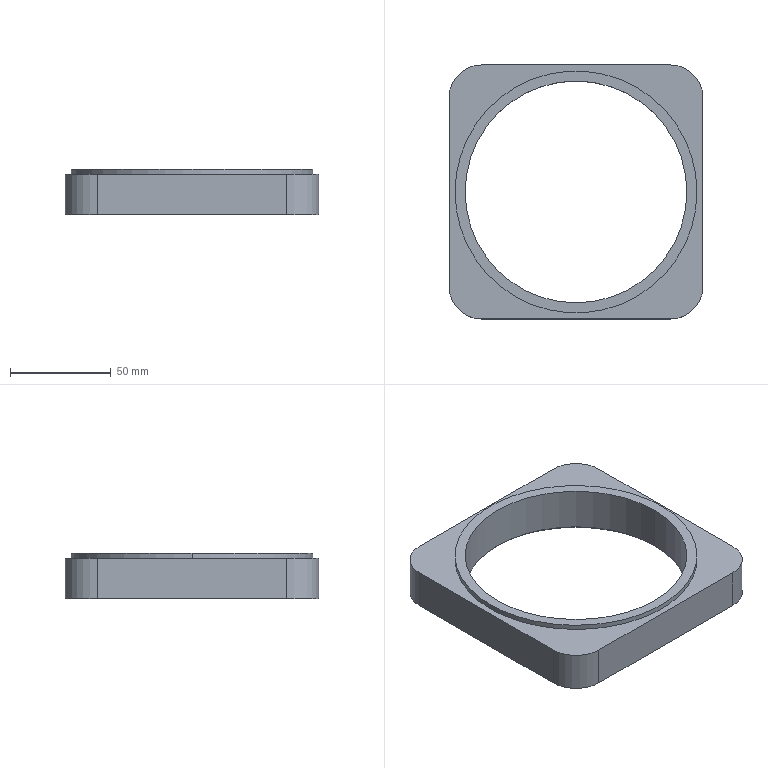Part | SolidWorks | features 3DProfileFeature 1, Chamfer 1, Extrusion 1, HoleWzd 1, ICE 1 | 1 solid | 33 faces | box 126 x 126 x 22.5 mm | volume 124484 mm3 | cylinder 16 | cone 10 | plane 7 | commonest cylinder face diameters 8.5 x8 32 x4 110 x2 120 x2
STEP:
#1=CARTESIAN_POINT('',(118.,63.,1.));
#2=VERTEX_POINT('',#1);
#3=CARTESIAN_POINT('',(8.,63.,1.));
#4=VERTEX_POINT('',#3);
#5=CARTESIAN_POINT('',(63.,63.,1.));
#6=DIRECTION('',(0.,0.,-1.));
#7=DIRECTION('',(1.,0.,0.));
#8=AXIS2_PLACEMENT_3D('',#5,#6,#7);
#9=CIRCLE('',#8,55.);
#10=EDGE_CURVE('',#2,#4,#9,.T.);
#11=ORIENTED_EDGE('',*,*,#10,.F.);
#12=CARTESIAN_POINT('',(119.,63.,0.));
#13=VERTEX_POINT('',#12);
#14=CARTESIAN_POINT('',(119.,63.,0.));
#15=DIRECTION('',(0.7071,0.,-0.7071));
#16=VECTOR('',#15,1000.);
#17=LINE('',#14,#16);
#18=EDGE_CURVE('',#2,#13,#17,.T.);
#19=ORIENTED_EDGE('',*,*,#18,.T.);
#20=CARTESIAN_POINT('',(7.,63.,0.));
#21=VERTEX_POINT('',#20);
#22=CARTESIAN_POINT('',(63.,63.,0.));
#23=DIRECTION('',(0.,0.,1.));
#24=DIRECTION('',(1.,0.,0.));
#25=AXIS2_PLACEMENT_3D('',#22,#23,#24);
#26=CIRCLE('',#25,56.);
#27=EDGE_CURVE('',#21,#13,#26,.T.);
#28=ORIENTED_EDGE('',*,*,#27,.F.);
#29=CARTESIAN_POINT('',(7.,63.,0.));
#30=DIRECTION('',(-0.7071,0.,-0.7071));
#31=VECTOR('',#30,1000.);
#32=LINE('',#29,#31);
#33=EDGE_CURVE('',#4,#21,#32,.T.);
#34=ORIENTED_EDGE('',*,*,#33,.F.);
#35=EDGE_LOOP('',(#11,#19,#28,#34));
#36=FACE_OUTER_BOUND('',#35,.T.);
#37=CARTESIAN_POINT('',(63.,63.,0.));
#38=DIRECTION('',(0.,0.,-1.));
#39=DIRECTION('',(-1.,0.,0.));
#40=AXIS2_PLACEMENT_3D('',#37,#38,#39);
#41=CONICAL_SURFACE('',#40,56.,0.7854);
#42=ADVANCED_FACE('',(#36),#41,.F.);
#43=CARTESIAN_POINT('',(114.25,110.,12.));
#44=VERTEX_POINT('',#43);
#45=CARTESIAN_POINT('',(105.75,110.,12.));
#46=VERTEX_POINT('',#45);
#47=CARTESIAN_POINT('',(110.,110.,12.));
#48=DIRECTION('',(0.,0.,-1.));
#49=DIRECTION('',(-1.,0.,0.));
#50=AXIS2_PLACEMENT_3D('',#47,#48,#49);
#51=CIRCLE('',#50,4.25);
#52=EDGE_CURVE('',#44,#46,#51,.T.);
#53=ORIENTED_EDGE('',*,*,#52,.F.);
#54=CARTESIAN_POINT('',(114.25,110.,0.));
#55=VERTEX_POINT('',#54);
#56=CARTESIAN_POINT('',(114.25,110.,0.));
#57=DIRECTION('',(0.,0.,-1.));
#58=VECTOR('',#57,1000.);
#59=LINE('',#56,#58);
#60=EDGE_CURVE('',#44,#55,#59,.T.);
#61=ORIENTED_EDGE('',*,*,#60,.T.);
#62=CARTESIAN_POINT('',(105.75,110.,0.));
#63=VERTEX_POINT('',#62);
#64=CARTESIAN_POINT('',(110.,110.,0.));
#65=DIRECTION('',(0.,0.,-1.));
#66=DIRECTION('',(-1.,0.,0.));
#67=AXIS2_PLACEMENT_3D('',#64,#65,#66);
#68=CIRCLE('',#67,4.25);
#69=EDGE_CURVE('',#55,#63,#68,.T.);
#70=ORIENTED_EDGE('',*,*,#69,.T.);
#71=CARTESIAN_POINT('',(105.75,110.,0.));
#72=DIRECTION('',(0.,0.,-1.));
#73=VECTOR('',#72,1000.);
#74=LINE('',#71,#73);
#75=EDGE_CURVE('',#46,#63,#74,.T.);
#76=ORIENTED_EDGE('',*,*,#75,.F.);
#77=EDGE_LOOP('',(#53,#61,#70,#76));
#78=FACE_OUTER_BOUND('',#77,.T.);
#79=CARTESIAN_POINT('',(110.,110.,0.));
#80=DIRECTION('',(0.,0.,-1.));
#81=DIRECTION('',(-1.,0.,0.));
#82=AXIS2_PLACEMENT_3D('',#79,#80,#81);
#83=CYLINDRICAL_SURFACE('',#82,4.25);
#84=ADVANCED_FACE('',(#78),#83,.F.);
#85=CARTESIAN_POINT('',(110.,110.,14.554));
#86=VERTEX_POINT('',#85);
#87=CARTESIAN_POINT('',(105.75,110.,12.));
#88=DIRECTION('',(-0.8572,0.,-0.515));
#89=VECTOR('',#88,1000.);
#90=LINE('',#87,#89);
#91=EDGE_CURVE('',#86,#46,#90,.T.);
#92=ORIENTED_EDGE('',*,*,#91,.F.);
#93=CARTESIAN_POINT('',(114.25,110.,12.));
#94=DIRECTION('',(0.8572,0.,-0.515));
#95=VECTOR('',#94,1000.);
#96=LINE('',#93,#95);
#97=EDGE_CURVE('',#86,#44,#96,.T.);
#98=ORIENTED_EDGE('',*,*,#97,.T.);
#99=ORIENTED_EDGE('',*,*,#52,.T.);
#100=EDGE_LOOP('',(#92,#98,#99));
#101=FACE_OUTER_BOUND('',#100,.T.);
#102=CARTESIAN_POINT('',(110.,110.,12.));
#103=DIRECTION('',(0.,0.,-1.));
#104=DIRECTION('',(-1.,0.,0.));
#105=AXIS2_PLACEMENT_3D('',#102,#103,#104);
#106=CONICAL_SURFACE('',#105,4.25,1.03);
#107=ADVANCED_FACE('',(#101),#106,.F.);
#108=CARTESIAN_POINT('',(20.25,110.,12.));
#109=VERTEX_POINT('',#108);
#110=CARTESIAN_POINT('',(11.75,110.,12.));
#111=VERTEX_POINT('',#110);
#112=CARTESIAN_POINT('',(16.,110.,12.));
#113=DIRECTION('',(0.,0.,-1.));
#114=DIRECTION('',(-1.,0.,0.));
#115=AXIS2_PLACEMENT_3D('',#112,#113,#114);
#116=CIRCLE('',#115,4.25);
#117=EDGE_CURVE('',#109,#111,#116,.T.);
#118=ORIENTED_EDGE('',*,*,#117,.F.);
#119=CARTESIAN_POINT('',(20.25,110.,0.));
#120=VERTEX_POINT('',#119);
#121=CARTESIAN_POINT('',(20.25,110.,0.));
#122=DIRECTION('',(0.,0.,-1.));
#123=VECTOR('',#122,1000.);
#124=LINE('',#121,#123);
#125=EDGE_CURVE('',#109,#120,#124,.T.);
#126=ORIENTED_EDGE('',*,*,#125,.T.);
#127=CARTESIAN_POINT('',(11.75,110.,0.));
#128=VERTEX_POINT('',#127);
#129=CARTESIAN_POINT('',(16.,110.,0.));
#130=DIRECTION('',(0.,0.,-1.));
#131=DIRECTION('',(-1.,0.,0.));
#132=AXIS2_PLACEMENT_3D('',#129,#130,#131);
#133=CIRCLE('',#132,4.25);
#134=EDGE_CURVE('',#120,#128,#133,.T.);
#135=ORIENTED_EDGE('',*,*,#134,.T.);
#136=CARTESIAN_POINT('',(11.75,110.,0.));
#137=DIRECTION('',(0.,0.,-1.));
#138=VECTOR('',#137,1000.);
#139=LINE('',#136,#138);
#140=EDGE_CURVE('',#111,#128,#139,.T.);
#141=ORIENTED_EDGE('',*,*,#140,.F.);
#142=EDGE_LOOP('',(#118,#126,#135,#141));
#143=FACE_OUTER_BOUND('',#142,.T.);
#144=CARTESIAN_POINT('',(16.,110.,0.));
#145=DIRECTION('',(0.,0.,-1.));
#146=DIRECTION('',(-1.,0.,0.));
#147=AXIS2_PLACEMENT_3D('',#144,#145,#146);
#148=CYLINDRICAL_SURFACE('',#147,4.25);
#149=ADVANCED_FACE('',(#143),#148,.F.);
#150=CARTESIAN_POINT('',(16.,110.,14.554));
#151=VERTEX_POINT('',#150);
#152=CARTESIAN_POINT('',(11.75,110.,12.));
#153=DIRECTION('',(-0.8572,0.,-0.515));
#154=VECTOR('',#153,1000.);
#155=LINE('',#152,#154);
#156=EDGE_CURVE('',#151,#111,#155,.T.);
#157=ORIENTED_EDGE('',*,*,#156,.F.);
#158=CARTESIAN_POINT('',(20.25,110.,12.));
#159=DIRECTION('',(0.8572,0.,-0.515));
#160=VECTOR('',#159,1000.);
#161=LINE('',#158,#160);
#162=EDGE_CURVE('',#151,#109,#161,.T.);
#163=ORIENTED_EDGE('',*,*,#162,.T.);
#164=ORIENTED_EDGE('',*,*,#117,.T.);
#165=EDGE_LOOP('',(#157,#163,#164));
#166=FACE_OUTER_BOUND('',#165,.T.);
#167=CARTESIAN_POINT('',(16.,110.,12.));
#168=DIRECTION('',(0.,0.,-1.));
#169=DIRECTION('',(-1.,0.,0.));
#170=AXIS2_PLACEMENT_3D('',#167,#168,#169);
#171=CONICAL_SURFACE('',#170,4.25,1.03);
#172=ADVANCED_FACE('',(#166),#171,.F.);
#173=CARTESIAN_POINT('',(20.25,16.,12.));
#174=VERTEX_POINT('',#173);
#175=CARTESIAN_POINT('',(11.75,16.,12.));
#176=VERTEX_POINT('',#175);
#177=CARTESIAN_POINT('',(16.,16.,12.));
#178=DIRECTION('',(0.,0.,-1.));
#179=DIRECTION('',(-1.,0.,0.));
#180=AXIS2_PLACEMENT_3D('',#177,#178,#179);
#181=CIRCLE('',#180,4.25);
#182=EDGE_CURVE('',#174,#176,#181,.T.);
#183=ORIENTED_EDGE('',*,*,#182,.F.);
#184=CARTESIAN_POINT('',(20.25,16.,0.));
#185=VERTEX_POINT('',#184);
#186=CARTESIAN_POINT('',(20.25,16.,0.));
#187=DIRECTION('',(0.,0.,-1.));
#188=VECTOR('',#187,1000.);
#189=LINE('',#186,#188);
#190=EDGE_CURVE('',#174,#185,#189,.T.);
#191=ORIENTED_EDGE('',*,*,#190,.T.);
#192=CARTESIAN_POINT('',(11.75,16.,0.));
#193=VERTEX_POINT('',#192);
#194=CARTESIAN_POINT('',(16.,16.,0.));
#195=DIRECTION('',(0.,0.,-1.));
#196=DIRECTION('',(-1.,0.,0.));
#197=AXIS2_PLACEMENT_3D('',#194,#195,#196);
#198=CIRCLE('',#197,4.25);
#199=EDGE_CURVE('',#185,#193,#198,.T.);
#200=ORIENTED_EDGE('',*,*,#199,.T.);
#201=CARTESIAN_POINT('',(11.75,16.,0.));
#202=DIRECTION('',(0.,0.,-1.));
#203=VECTOR('',#202,1000.);
#204=LINE('',#201,#203);
#205=EDGE_CURVE('',#176,#193,#204,.T.);
#206=ORIENTED_EDGE('',*,*,#205,.F.);
#207=EDGE_LOOP('',(#183,#191,#200,#206));
#208=FACE_OUTER_BOUND('',#207,.T.);
#209=CARTESIAN_POINT('',(16.,16.,0.));
#210=DIRECTION('',(0.,0.,-1.));
#211=DIRECTION('',(-1.,0.,0.));
#212=AXIS2_PLACEMENT_3D('',#209,#210,#211);
#213=CYLINDRICAL_SURFACE('',#212,4.25);
#214=ADVANCED_FACE('',(#208),#213,.F.);
#215=CARTESIAN_POINT('',(16.,16.,14.554));
#216=VERTEX_POINT('',#215);
#217=CARTESIAN_POINT('',(11.75,16.,12.));
#218=DIRECTION('',(-0.8572,0.,-0.515));
#219=VECTOR('',#218,1000.);
#220=LINE('',#217,#219);
#221=EDGE_CURVE('',#216,#176,#220,.T.);
#222=ORIENTED_EDGE('',*,*,#221,.F.);
#223=CARTESIAN_POINT('',(20.25,16.,12.));
#224=DIRECTION('',(0.8572,0.,-0.515));
#225=VECTOR('',#224,1000.);
#226=LINE('',#223,#225);
#227=EDGE_CURVE('',#216,#174,#226,.T.);
#228=ORIENTED_EDGE('',*,*,#227,.T.);
#229=ORIENTED_EDGE('',*,*,#182,.T.);
#230=EDGE_LOOP('',(#222,#228,#229));
#231=FACE_OUTER_BOUND('',#230,.T.);
#232=CARTESIAN_POINT('',(16.,16.,12.));
#233=DIRECTION('',(0.,0.,-1.));
#234=DIRECTION('',(-1.,0.,0.));
#235=AXIS2_PLACEMENT_3D('',#232,#233,#234);
#236=CONICAL_SURFACE('',#235,4.25,1.03);
#237=ADVANCED_FACE('',(#231),#236,.F.);
#238=CARTESIAN_POINT('',(114.25,16.,12.));
#239=VERTEX_POINT('',#238);
#240=CARTESIAN_POINT('',(105.75,16.,12.));
#241=VERTEX_POINT('',#240);
#242=CARTESIAN_POINT('',(110.,16.,12.));
#243=DIRECTION('',(0.,0.,-1.));
#244=DIRECTION('',(-1.,0.,0.));
#245=AXIS2_PLACEMENT_3D('',#242,#243,#244);
#246=CIRCLE('',#245,4.25);
#247=EDGE_CURVE('',#239,#241,#246,.T.);
#248=ORIENTED_EDGE('',*,*,#247,.F.);
#249=CARTESIAN_POINT('',(114.25,16.,0.));
#250=VERTEX_POINT('',#249);
#251=CARTESIAN_POINT('',(114.25,16.,0.));
#252=DIRECTION('',(0.,0.,-1.));
#253=VECTOR('',#252,1000.);
#254=LINE('',#251,#253);
#255=EDGE_CURVE('',#239,#250,#254,.T.);
#256=ORIENTED_EDGE('',*,*,#255,.T.);
#257=CARTESIAN_POINT('',(105.75,16.,0.));
#258=VERTEX_POINT('',#257);
#259=CARTESIAN_POINT('',(110.,16.,0.));
#260=DIRECTION('',(0.,0.,-1.));
#261=DIRECTION('',(-1.,0.,0.));
#262=AXIS2_PLACEMENT_3D('',#259,#260,#261);
#263=CIRCLE('',#262,4.25);
#264=EDGE_CURVE('',#250,#258,#263,.T.);
#265=ORIENTED_EDGE('',*,*,#264,.T.);
#266=CARTESIAN_POINT('',(105.75,16.,0.));
#267=DIRECTION('',(0.,0.,-1.));
#268=VECTOR('',#267,1000.);
#269=LINE('',#266,#268);
#270=EDGE_CURVE('',#241,#258,#269,.T.);
#271=ORIENTED_EDGE('',*,*,#270,.F.);
#272=EDGE_LOOP('',(#248,#256,#265,#271));
#273=FACE_OUTER_BOUND('',#272,.T.);
#274=CARTESIAN_POINT('',(110.,16.,0.));
#275=DIRECTION('',(0.,0.,-1.));
#276=DIRECTION('',(-1.,0.,0.));
#277=AXIS2_PLACEMENT_3D('',#274,#275,#276);
#278=CYLINDRICAL_SURFACE('',#277,4.25);
#279=ADVANCED_FACE('',(#273),#278,.F.);
#280=CARTESIAN_POINT('',(110.,16.,14.554));
#281=VERTEX_POINT('',#280);
#282=CARTESIAN_POINT('',(105.75,16.,12.));
#283=DIRECTION('',(-0.8572,0.,-0.515));
#284=VECTOR('',#283,1000.);
#285=LINE('',#282,#284);
#286=EDGE_CURVE('',#281,#241,#285,.T.);
#287=ORIENTED_EDGE('',*,*,#286,.F.);
#288=CARTESIAN_POINT('',(114.25,16.,12.));
#289=DIRECTION('',(0.8572,0.,-0.515));
#290=VECTOR('',#289,1000.);
#291=LINE('',#288,#290);
#292=EDGE_CURVE('',#281,#239,#291,.T.);
#293=ORIENTED_EDGE('',*,*,#292,.T.);
#294=ORIENTED_EDGE('',*,*,#247,.T.);
#295=EDGE_LOOP('',(#287,#293,#294));
#296=FACE_OUTER_BOUND('',#295,.T.);
#297=CARTESIAN_POINT('',(110.,16.,12.));
#298=DIRECTION('',(0.,0.,-1.));
#299=DIRECTION('',(-1.,0.,0.));
#300=AXIS2_PLACEMENT_3D('',#297,#298,#299);
#301=CONICAL_SURFACE('',#300,4.25,1.03);
#302=ADVANCED_FACE('',(#296),#301,.F.);
#303=CARTESIAN_POINT('',(123.,63.,22.5));
#304=VERTEX_POINT('',#303);
#305=CARTESIAN_POINT('',(3.,63.,22.5));
#306=VERTEX_POINT('',#305);
#307=CARTESIAN_POINT('',(63.,63.,22.5));
#308=DIRECTION('',(0.,0.,1.));
#309=DIRECTION('',(1.,0.,0.));
#310=AXIS2_PLACEMENT_3D('',#307,#308,#309);
#311=CIRCLE('',#310,60.);
#312=EDGE_CURVE('',#304,#306,#311,.T.);
#313=ORIENTED_EDGE('',*,*,#312,.F.);
#314=CARTESIAN_POINT('',(123.,63.,20.));
#315=VERTEX_POINT('',#314);
#316=CARTESIAN_POINT('',(123.,63.,22.5));
#317=DIRECTION('',(0.,0.,-1.));
#318=VECTOR('',#317,1000.);
#319=LINE('',#316,#318);
#320=EDGE_CURVE('',#304,#315,#319,.T.);
#321=ORIENTED_EDGE('',*,*,#320,.T.);
#322=CARTESIAN_POINT('',(3.,63.,20.));
#323=VERTEX_POINT('',#322);
#324=CARTESIAN_POINT('',(63.,63.,20.));
#325=DIRECTION('',(0.,0.,1.));
#326=DIRECTION('',(1.,0.,0.));
#327=AXIS2_PLACEMENT_3D('',#324,#325,#326);
#328=CIRCLE('',#327,60.);
#329=EDGE_CURVE('',#315,#323,#328,.T.);
#330=ORIENTED_EDGE('',*,*,#329,.T.);
#331=CARTESIAN_POINT('',(3.,63.,22.5));
#332=DIRECTION('',(0.,0.,-1.));
#333=VECTOR('',#332,1000.);
#334=LINE('',#331,#333);
#335=EDGE_CURVE('',#306,#323,#334,.T.);
#336=ORIENTED_EDGE('',*,*,#335,.F.);
#337=EDGE_LOOP('',(#313,#321,#330,#336));
#338=FACE_OUTER_BOUND('',#337,.T.);
#339=CARTESIAN_POINT('',(63.,63.,22.5));
#340=DIRECTION('',(0.,0.,-1.));
#341=DIRECTION('',(-1.,0.,0.));
#342=AXIS2_PLACEMENT_3D('',#339,#340,#341);
#343=CYLINDRICAL_SURFACE('',#342,60.);
#344=ADVANCED_FACE('',(#338),#343,.T.);
#345=CARTESIAN_POINT('',(8.,63.,22.5));
#346=VERTEX_POINT('',#345);
#347=CARTESIAN_POINT('',(118.,63.,22.5));
#348=VERTEX_POINT('',#347);
#349=CARTESIAN_POINT('',(63.,63.,22.5));
#350=DIRECTION('',(0.,0.,1.));
#351=DIRECTION('',(1.,0.,0.));
#352=AXIS2_PLACEMENT_3D('',#349,#350,#351);
#353=CIRCLE('',#352,55.);
#354=EDGE_CURVE('',#346,#348,#353,.T.);
#355=ORIENTED_EDGE('',*,*,#354,.T.);
#356=CARTESIAN_POINT('',(118.,63.,20.));
#357=DIRECTION('',(0.,0.,-1.));
#358=VECTOR('',#357,1000.);
#359=LINE('',#356,#358);
#360=EDGE_CURVE('',#348,#2,#359,.T.);
#361=ORIENTED_EDGE('',*,*,#360,.T.);
#362=ORIENTED_EDGE('',*,*,#10,.T.);
#363=CARTESIAN_POINT('',(8.,63.,20.));
#364=DIRECTION('',(0.,0.,-1.));
#365=VECTOR('',#364,1000.);
#366=LINE('',#363,#365);
#367=EDGE_CURVE('',#346,#4,#366,.T.);
#368=ORIENTED_EDGE('',*,*,#367,.F.);
#369=EDGE_LOOP('',(#355,#361,#362,#368));
#370=FACE_OUTER_BOUND('',#369,.T.);
#371=CARTESIAN_POINT('',(63.,63.,20.));
#372=DIRECTION('',(0.,0.,-1.));
#373=DIRECTION('',(-1.,0.,0.));
#374=AXIS2_PLACEMENT_3D('',#371,#372,#373);
#375=CYLINDRICAL_SURFACE('',#374,55.);
#376=ADVANCED_FACE('',(#370),#375,.F.);
#377=CARTESIAN_POINT('',(0.,16.,20.));
#378=VERTEX_POINT('',#377);
#379=CARTESIAN_POINT('',(16.,0.,20.));
#380=VERTEX_POINT('',#379);
#381=CARTESIAN_POINT('',(16.,16.,20.));
#382=DIRECTION('',(0.,0.,1.));
#383=DIRECTION('',(1.,0.,0.));
#384=AXIS2_PLACEMENT_3D('',#381,#382,#383);
#385=CIRCLE('',#384,16.);
#386=EDGE_CURVE('',#378,#380,#385,.T.);
#387=ORIENTED_EDGE('',*,*,#386,.T.);
#388=CARTESIAN_POINT('',(110.,0.,20.));
#389=VERTEX_POINT('',#388);
#390=CARTESIAN_POINT('',(16.,0.,20.));
#391=DIRECTION('',(1.,0.,0.));
#392=VECTOR('',#391,1000.);
#393=LINE('',#390,#392);
#394=EDGE_CURVE('',#380,#389,#393,.T.);
#395=ORIENTED_EDGE('',*,*,#394,.T.);
#396=CARTESIAN_POINT('',(126.,16.,20.));
#397=VERTEX_POINT('',#396);
#398=CARTESIAN_POINT('',(110.,16.,20.));
#399=DIRECTION('',(0.,0.,1.));
#400=DIRECTION('',(-1.,0.,0.));
#401=AXIS2_PLACEMENT_3D('',#398,#399,#400);
#402=CIRCLE('',#401,16.);
#403=EDGE_CURVE('',#389,#397,#402,.T.);
#404=ORIENTED_EDGE('',*,*,#403,.T.);
#405=CARTESIAN_POINT('',(126.,110.,20.));
#406=VERTEX_POINT('',#405);
#407=CARTESIAN_POINT('',(126.,16.,20.));
#408=DIRECTION('',(0.,1.,0.));
#409=VECTOR('',#408,1000.);
#410=LINE('',#407,#409);
#411=EDGE_CURVE('',#397,#406,#410,.T.);
#412=ORIENTED_EDGE('',*,*,#411,.T.);
#413=CARTESIAN_POINT('',(110.,126.,20.));
#414=VERTEX_POINT('',#413);
#415=CARTESIAN_POINT('',(110.,110.,20.));
#416=DIRECTION('',(0.,0.,1.));
#417=DIRECTION('',(1.,0.,0.));
#418=AXIS2_PLACEMENT_3D('',#415,#416,#417);
#419=CIRCLE('',#418,16.);
#420=EDGE_CURVE('',#406,#414,#419,.T.);
#421=ORIENTED_EDGE('',*,*,#420,.T.);
#422=CARTESIAN_POINT('',(16.,126.,20.));
#423=VERTEX_POINT('',#422);
#424=CARTESIAN_POINT('',(110.,126.,20.));
#425=DIRECTION('',(-1.,0.,0.));
#426=VECTOR('',#425,1000.);
#427=LINE('',#424,#426);
#428=EDGE_CURVE('',#414,#423,#427,.T.);
#429=ORIENTED_EDGE('',*,*,#428,.T.);
#430=CARTESIAN_POINT('',(0.,110.,20.));
#431=VERTEX_POINT('',#430);
#432=CARTESIAN_POINT('',(16.,110.,20.));
#433=DIRECTION('',(0.,0.,1.));
#434=DIRECTION('',(-1.,0.,0.));
#435=AXIS2_PLACEMENT_3D('',#432,#433,#434);
#436=CIRCLE('',#435,16.);
#437=EDGE_CURVE('',#423,#431,#436,.T.);
#438=ORIENTED_EDGE('',*,*,#437,.T.);
#439=CARTESIAN_POINT('',(0.,110.,20.));
#440=DIRECTION('',(0.,-1.,0.));
#441=VECTOR('',#440,1000.);
#442=LINE('',#439,#441);
#443=EDGE_CURVE('',#431,#378,#442,.T.);
#444=ORIENTED_EDGE('',*,*,#443,.T.);
#445=EDGE_LOOP('',(#387,#395,#404,#412,#421,#429,#438,#444));
#446=FACE_OUTER_BOUND('',#445,.T.);
#447=CARTESIAN_POINT('',(63.,63.,20.));
#448=DIRECTION('',(0.,0.,1.));
#449=DIRECTION('',(1.,0.,0.));
#450=AXIS2_PLACEMENT_3D('',#447,#448,#449);
#451=CIRCLE('',#450,60.);
#452=EDGE_CURVE('',#323,#315,#451,.T.);
#453=ORIENTED_EDGE('',*,*,#452,.F.);
#454=ORIENTED_EDGE('',*,*,#329,.F.);
#455=EDGE_LOOP('',(#453,#454));
#456=FACE_BOUND('',#455,.T.);
#457=CARTESIAN_POINT('',(16.,16.,20.));
#458=DIRECTION('',(0.,0.,1.));
#459=DIRECTION('',(1.,0.,0.));
#460=AXIS2_PLACEMENT_3D('',#457,#458,#459);
#461=PLANE('',#460);
#462=ADVANCED_FACE('',(#446,#456),#461,.T.);
#463=ORIENTED_EDGE('',*,*,#27,.T.);
#464=CARTESIAN_POINT('',(63.,63.,0.));
#465=DIRECTION('',(0.,0.,1.));
#466=DIRECTION('',(1.,0.,0.));
#467=AXIS2_PLACEMENT_3D('',#464,#465,#466);
#468=CIRCLE('',#467,56.);
#469=EDGE_CURVE('',#13,#21,#468,.T.);
#470=ORIENTED_EDGE('',*,*,#469,.T.);
#471=EDGE_LOOP('',(#463,#470));
#472=FACE_BOUND('',#471,.T.);
#473=CARTESIAN_POINT('',(110.,110.,0.));
#474=DIRECTION('',(0.,0.,-1.));
#475=DIRECTION('',(-1.,0.,0.));
#476=AXIS2_PLACEMENT_3D('',#473,#474,#475);
#477=CIRCLE('',#476,4.25);
#478=EDGE_CURVE('',#63,#55,#477,.T.);
#479=ORIENTED_EDGE('',*,*,#478,.F.);
#480=ORIENTED_EDGE('',*,*,#69,.F.);
#481=EDGE_LOOP('',(#479,#480));
#482=FACE_BOUND('',#481,.T.);
#483=CARTESIAN_POINT('',(16.,110.,0.));
#484=DIRECTION('',(0.,0.,-1.));
#485=DIRECTION('',(-1.,0.,0.));
#486=AXIS2_PLACEMENT_3D('',#483,#484,#485);
#487=CIRCLE('',#486,4.25);
#488=EDGE_CURVE('',#128,#120,#487,.T.);
#489=ORIENTED_EDGE('',*,*,#488,.F.);
#490=ORIENTED_EDGE('',*,*,#134,.F.);
#491=EDGE_LOOP('',(#489,#490));
#492=FACE_BOUND('',#491,.T.);
#493=CARTESIAN_POINT('',(16.,16.,0.));
#494=DIRECTION('',(0.,0.,-1.));
#495=DIRECTION('',(-1.,0.,0.));
#496=AXIS2_PLACEMENT_3D('',#493,#494,#495);
#497=CIRCLE('',#496,4.25);
#498=EDGE_CURVE('',#193,#185,#497,.T.);
#499=ORIENTED_EDGE('',*,*,#498,.F.);
#500=ORIENTED_EDGE('',*,*,#199,.F.);
#501=EDGE_LOOP('',(#499,#500));
#502=FACE_BOUND('',#501,.T.);
#503=CARTESIAN_POINT('',(110.,16.,0.));
#504=DIRECTION('',(0.,0.,-1.));
#505=DIRECTION('',(-1.,0.,0.));
#506=AXIS2_PLACEMENT_3D('',#503,#504,#505);
#507=CIRCLE('',#506,4.25);
#508=EDGE_CURVE('',#258,#250,#507,.T.);
#509=ORIENTED_EDGE('',*,*,#508,.F.);
#510=ORIENTED_EDGE('',*,*,#264,.F.);
#511=EDGE_LOOP('',(#509,#510));
#512=FACE_BOUND('',#511,.T.);
#513=CARTESIAN_POINT('',(0.,16.,0.));
#514=VERTEX_POINT('',#513);
#515=CARTESIAN_POINT('',(16.,0.,0.));
#516=VERTEX_POINT('',#515);
#517=CARTESIAN_POINT('',(16.,16.,0.));
#518=DIRECTION('',(0.,0.,1.));
#519=DIRECTION('',(1.,0.,0.));
#520=AXIS2_PLACEMENT_3D('',#517,#518,#519);
#521=CIRCLE('',#520,16.);
#522=EDGE_CURVE('',#514,#516,#521,.T.);
#523=ORIENTED_EDGE('',*,*,#522,.F.);
#524=CARTESIAN_POINT('',(0.,110.,0.));
#525=VERTEX_POINT('',#524);
#526=CARTESIAN_POINT('',(0.,110.,0.));
#527=DIRECTION('',(0.,-1.,0.));
#528=VECTOR('',#527,1000.);
#529=LINE('',#526,#528);
#530=EDGE_CURVE('',#525,#514,#529,.T.);
#531=ORIENTED_EDGE('',*,*,#530,.F.);
#532=CARTESIAN_POINT('',(16.,126.,0.));
#533=VERTEX_POINT('',#532);
#534=CARTESIAN_POINT('',(16.,110.,0.));
#535=DIRECTION('',(0.,0.,1.));
#536=DIRECTION('',(-1.,0.,0.));
#537=AXIS2_PLACEMENT_3D('',#534,#535,#536);
#538=CIRCLE('',#537,16.);
#539=EDGE_CURVE('',#533,#525,#538,.T.);
#540=ORIENTED_EDGE('',*,*,#539,.F.);
#541=CARTESIAN_POINT('',(110.,126.,0.));
#542=VERTEX_POINT('',#541);
#543=CARTESIAN_POINT('',(110.,126.,0.));
#544=DIRECTION('',(-1.,0.,0.));
#545=VECTOR('',#544,1000.);
#546=LINE('',#543,#545);
#547=EDGE_CURVE('',#542,#533,#546,.T.);
#548=ORIENTED_EDGE('',*,*,#547,.F.);
#549=CARTESIAN_POINT('',(126.,110.,0.));
#550=VERTEX_POINT('',#549);
#551=CARTESIAN_POINT('',(110.,110.,0.));
#552=DIRECTION('',(0.,0.,1.));
#553=DIRECTION('',(1.,0.,0.));
#554=AXIS2_PLACEMENT_3D('',#551,#552,#553);
#555=CIRCLE('',#554,16.);
#556=EDGE_CURVE('',#550,#542,#555,.T.);
#557=ORIENTED_EDGE('',*,*,#556,.F.);
#558=CARTESIAN_POINT('',(126.,16.,0.));
#559=VERTEX_POINT('',#558);
#560=CARTESIAN_POINT('',(126.,16.,0.));
#561=DIRECTION('',(0.,1.,0.));
#562=VECTOR('',#561,1000.);
#563=LINE('',#560,#562);
#564=EDGE_CURVE('',#559,#550,#563,.T.);
#565=ORIENTED_EDGE('',*,*,#564,.F.);
#566=CARTESIAN_POINT('',(110.,0.,0.));
#567=VERTEX_POINT('',#566);
#568=CARTESIAN_POINT('',(110.,16.,0.));
#569=DIRECTION('',(0.,0.,1.));
#570=DIRECTION('',(-1.,0.,0.));
#571=AXIS2_PLACEMENT_3D('',#568,#569,#570);
#572=CIRCLE('',#571,16.);
#573=EDGE_CURVE('',#567,#559,#572,.T.);
#574=ORIENTED_EDGE('',*,*,#573,.F.);
#575=CARTESIAN_POINT('',(16.,0.,0.));
#576=DIRECTION('',(1.,0.,0.));
#577=VECTOR('',#576,1000.);
#578=LINE('',#575,#577);
#579=EDGE_CURVE('',#516,#567,#578,.T.);
#580=ORIENTED_EDGE('',*,*,#579,.F.);
#581=EDGE_LOOP('',(#523,#531,#540,#548,#557,#565,#574,#580));
#582=FACE_OUTER_BOUND('',#581,.T.);
#583=CARTESIAN_POINT('',(16.,16.,0.));
#584=DIRECTION('',(0.,0.,1.));
#585=DIRECTION('',(1.,0.,0.));
#586=AXIS2_PLACEMENT_3D('',#583,#584,#585);
#587=PLANE('',#586);
#588=ADVANCED_FACE('',(#472,#482,#492,#502,#512,#582),#587,.F.);
#589=ORIENTED_EDGE('',*,*,#522,.T.);
#590=CARTESIAN_POINT('',(16.,0.,20.));
#591=DIRECTION('',(0.,0.,-1.));
#592=VECTOR('',#591,1000.);
#593=LINE('',#590,#592);
#594=EDGE_CURVE('',#380,#516,#593,.T.);
#595=ORIENTED_EDGE('',*,*,#594,.F.);
#596=ORIENTED_EDGE('',*,*,#386,.F.);
#597=CARTESIAN_POINT('',(0.,16.,20.));
#598=DIRECTION('',(0.,0.,-1.));
#599=VECTOR('',#598,1000.);
#600=LINE('',#597,#599);
#601=EDGE_CURVE('',#378,#514,#600,.T.);
#602=ORIENTED_EDGE('',*,*,#601,.T.);
#603=EDGE_LOOP('',(#589,#595,#596,#602));
#604=FACE_OUTER_BOUND('',#603,.T.);
#605=CARTESIAN_POINT('',(16.,16.,20.));
#606=DIRECTION('',(0.,0.,-1.));
#607=DIRECTION('',(-1.,0.,0.));
#608=AXIS2_PLACEMENT_3D('',#605,#606,#607);
#609=CYLINDRICAL_SURFACE('',#608,16.);
#610=ADVANCED_FACE('',(#604),#609,.T.);
#611=ORIENTED_EDGE('',*,*,#579,.T.);
#612=CARTESIAN_POINT('',(110.,0.,20.));
#613=DIRECTION('',(0.,0.,-1.));
#614=VECTOR('',#613,1000.);
#615=LINE('',#612,#614);
#616=EDGE_CURVE('',#389,#567,#615,.T.);
#617=ORIENTED_EDGE('',*,*,#616,.F.);
#618=ORIENTED_EDGE('',*,*,#394,.F.);
#619=ORIENTED_EDGE('',*,*,#594,.T.);
#620=EDGE_LOOP('',(#611,#617,#618,#619));
#621=FACE_OUTER_BOUND('',#620,.T.);
#622=CARTESIAN_POINT('',(16.,0.,20.));
#623=DIRECTION('',(0.,1.,0.));
#624=DIRECTION('',(0.,0.,1.));
#625=AXIS2_PLACEMENT_3D('',#622,#623,#624);
#626=PLANE('',#625);
#627=ADVANCED_FACE('',(#621),#626,.F.);
#628=ORIENTED_EDGE('',*,*,#573,.T.);
#629=CARTESIAN_POINT('',(126.,16.,20.));
#630=DIRECTION('',(0.,0.,-1.));
#631=VECTOR('',#630,1000.);
#632=LINE('',#629,#631);
#633=EDGE_CURVE('',#397,#559,#632,.T.);
#634=ORIENTED_EDGE('',*,*,#633,.F.);
#635=ORIENTED_EDGE('',*,*,#403,.F.);
#636=ORIENTED_EDGE('',*,*,#616,.T.);
#637=EDGE_LOOP('',(#628,#634,#635,#636));
#638=FACE_OUTER_BOUND('',#637,.T.);
#639=CARTESIAN_POINT('',(110.,16.,20.));
#640=DIRECTION('',(0.,0.,-1.));
#641=DIRECTION('',(-1.,0.,0.));
#642=AXIS2_PLACEMENT_3D('',#639,#640,#641);
#643=CYLINDRICAL_SURFACE('',#642,16.);
#644=ADVANCED_FACE('',(#638),#643,.T.);
#645=ORIENTED_EDGE('',*,*,#564,.T.);
#646=CARTESIAN_POINT('',(126.,110.,20.));
#647=DIRECTION('',(0.,0.,-1.));
#648=VECTOR('',#647,1000.);
#649=LINE('',#646,#648);
#650=EDGE_CURVE('',#406,#550,#649,.T.);
#651=ORIENTED_EDGE('',*,*,#650,.F.);
#652=ORIENTED_EDGE('',*,*,#411,.F.);
#653=ORIENTED_EDGE('',*,*,#633,.T.);
#654=EDGE_LOOP('',(#645,#651,#652,#653));
#655=FACE_OUTER_BOUND('',#654,.T.);
#656=CARTESIAN_POINT('',(126.,16.,20.));
#657=DIRECTION('',(-1.,0.,0.));
#658=DIRECTION('',(0.,0.,1.));
#659=AXIS2_PLACEMENT_3D('',#656,#657,#658);
#660=PLANE('',#659);
#661=ADVANCED_FACE('',(#655),#660,.F.);
#662=ORIENTED_EDGE('',*,*,#556,.T.);
#663=CARTESIAN_POINT('',(110.,126.,20.));
#664=DIRECTION('',(0.,0.,-1.));
#665=VECTOR('',#664,1000.);
#666=LINE('',#663,#665);
#667=EDGE_CURVE('',#414,#542,#666,.T.);
#668=ORIENTED_EDGE('',*,*,#667,.F.);
#669=ORIENTED_EDGE('',*,*,#420,.F.);
#670=ORIENTED_EDGE('',*,*,#650,.T.);
#671=EDGE_LOOP('',(#662,#668,#669,#670));
#672=FACE_OUTER_BOUND('',#671,.T.);
#673=CARTESIAN_POINT('',(110.,110.,20.));
#674=DIRECTION('',(0.,0.,-1.));
#675=DIRECTION('',(-1.,0.,0.));
#676=AXIS2_PLACEMENT_3D('',#673,#674,#675);
#677=CYLINDRICAL_SURFACE('',#676,16.);
#678=ADVANCED_FACE('',(#672),#677,.T.);
#679=ORIENTED_EDGE('',*,*,#547,.T.);
#680=CARTESIAN_POINT('',(16.,126.,20.));
#681=DIRECTION('',(0.,0.,-1.));
#682=VECTOR('',#681,1000.);
#683=LINE('',#680,#682);
#684=EDGE_CURVE('',#423,#533,#683,.T.);
#685=ORIENTED_EDGE('',*,*,#684,.F.);
#686=ORIENTED_EDGE('',*,*,#428,.F.);
#687=ORIENTED_EDGE('',*,*,#667,.T.);
#688=EDGE_LOOP('',(#679,#685,#686,#687));
#689=FACE_OUTER_BOUND('',#688,.T.);
#690=CARTESIAN_POINT('',(110.,126.,20.));
#691=DIRECTION('',(0.,-1.,0.));
#692=DIRECTION('',(0.,0.,-1.));
#693=AXIS2_PLACEMENT_3D('',#690,#691,#692);
#694=PLANE('',#693);
#695=ADVANCED_FACE('',(#689),#694,.F.);
#696=ORIENTED_EDGE('',*,*,#539,.T.);
#697=CARTESIAN_POINT('',(0.,110.,20.));
#698=DIRECTION('',(0.,0.,-1.));
#699=VECTOR('',#698,1000.);
#700=LINE('',#697,#699);
#701=EDGE_CURVE('',#431,#525,#700,.T.);
#702=ORIENTED_EDGE('',*,*,#701,.F.);
#703=ORIENTED_EDGE('',*,*,#437,.F.);
#704=ORIENTED_EDGE('',*,*,#684,.T.);
#705=EDGE_LOOP('',(#696,#702,#703,#704));
#706=FACE_OUTER_BOUND('',#705,.T.);
#707=CARTESIAN_POINT('',(16.,110.,20.));
#708=DIRECTION('',(0.,0.,-1.));
#709=DIRECTION('',(-1.,0.,0.));
#710=AXIS2_PLACEMENT_3D('',#707,#708,#709);
#711=CYLINDRICAL_SURFACE('',#710,16.);
#712=ADVANCED_FACE('',(#706),#711,.T.);
#713=ORIENTED_EDGE('',*,*,#530,.T.);
#714=ORIENTED_EDGE('',*,*,#601,.F.);
#715=ORIENTED_EDGE('',*,*,#443,.F.);
#716=ORIENTED_EDGE('',*,*,#701,.T.);
#717=EDGE_LOOP('',(#713,#714,#715,#716));
#718=FACE_OUTER_BOUND('',#717,.T.);
#719=CARTESIAN_POINT('',(0.,110.,20.));
#720=DIRECTION('',(1.,0.,0.));
#721=DIRECTION('',(0.,0.,-1.));
#722=AXIS2_PLACEMENT_3D('',#719,#720,#721);
#723=PLANE('',#722);
#724=ADVANCED_FACE('',(#718),#723,.F.);
#725=ORIENTED_EDGE('',*,*,#360,.F.);
#726=CARTESIAN_POINT('',(63.,63.,22.5));
#727=DIRECTION('',(0.,0.,1.));
#728=DIRECTION('',(1.,0.,0.));
#729=AXIS2_PLACEMENT_3D('',#726,#727,#728);
#730=CIRCLE('',#729,55.);
#731=EDGE_CURVE('',#348,#346,#730,.T.);
#732=ORIENTED_EDGE('',*,*,#731,.T.);
#733=ORIENTED_EDGE('',*,*,#367,.T.);
#734=CARTESIAN_POINT('',(63.,63.,1.));
#735=DIRECTION('',(0.,0.,-1.));
#736=DIRECTION('',(1.,0.,0.));
#737=AXIS2_PLACEMENT_3D('',#734,#735,#736);
#738=CIRCLE('',#737,55.);
#739=EDGE_CURVE('',#4,#2,#738,.T.);
#740=ORIENTED_EDGE('',*,*,#739,.T.);
#741=EDGE_LOOP('',(#725,#732,#733,#740));
#742=FACE_OUTER_BOUND('',#741,.T.);
#743=CARTESIAN_POINT('',(63.,63.,20.));
#744=DIRECTION('',(0.,0.,-1.));
#745=DIRECTION('',(-1.,0.,0.));
#746=AXIS2_PLACEMENT_3D('',#743,#744,#745);
#747=CYLINDRICAL_SURFACE('',#746,55.);
#748=ADVANCED_FACE('',(#742),#747,.F.);
#749=CARTESIAN_POINT('',(63.,63.,22.5));
#750=DIRECTION('',(0.,0.,1.));
#751=DIRECTION('',(1.,0.,0.));
#752=AXIS2_PLACEMENT_3D('',#749,#750,#751);
#753=CIRCLE('',#752,60.);
#754=EDGE_CURVE('',#306,#304,#753,.T.);
#755=ORIENTED_EDGE('',*,*,#754,.T.);
#756=ORIENTED_EDGE('',*,*,#312,.T.);
#757=EDGE_LOOP('',(#755,#756));
#758=FACE_OUTER_BOUND('',#757,.T.);
#759=ORIENTED_EDGE('',*,*,#354,.F.);
#760=ORIENTED_EDGE('',*,*,#731,.F.);
#761=EDGE_LOOP('',(#759,#760));
#762=FACE_BOUND('',#761,.T.);
#763=CARTESIAN_POINT('',(63.,63.,22.5));
#764=DIRECTION('',(0.,0.,1.));
#765=DIRECTION('',(1.,0.,0.));
#766=AXIS2_PLACEMENT_3D('',#763,#764,#765);
#767=PLANE('',#766);
#768=ADVANCED_FACE('',(#758,#762),#767,.T.);
#769=ORIENTED_EDGE('',*,*,#320,.F.);
#770=ORIENTED_EDGE('',*,*,#754,.F.);
#771=ORIENTED_EDGE('',*,*,#335,.T.);
#772=ORIENTED_EDGE('',*,*,#452,.T.);
#773=EDGE_LOOP('',(#769,#770,#771,#772));
#774=FACE_OUTER_BOUND('',#773,.T.);
#775=CARTESIAN_POINT('',(63.,63.,22.5));
#776=DIRECTION('',(0.,0.,-1.));
#777=DIRECTION('',(-1.,0.,0.));
#778=AXIS2_PLACEMENT_3D('',#775,#776,#777);
#779=CYLINDRICAL_SURFACE('',#778,60.);
#780=ADVANCED_FACE('',(#774),#779,.T.);
#781=ORIENTED_EDGE('',*,*,#292,.F.);
#782=ORIENTED_EDGE('',*,*,#286,.T.);
#783=CARTESIAN_POINT('',(110.,16.,12.));
#784=DIRECTION('',(0.,0.,-1.));
#785=DIRECTION('',(-1.,0.,0.));
#786=AXIS2_PLACEMENT_3D('',#783,#784,#785);
#787=CIRCLE('',#786,4.25);
#788=EDGE_CURVE('',#241,#239,#787,.T.);
#789=ORIENTED_EDGE('',*,*,#788,.T.);
#790=EDGE_LOOP('',(#781,#782,#789));
#791=FACE_OUTER_BOUND('',#790,.T.);
#792=CARTESIAN_POINT('',(110.,16.,12.));
#793=DIRECTION('',(0.,0.,-1.));
#794=DIRECTION('',(-1.,0.,0.));
#795=AXIS2_PLACEMENT_3D('',#792,#793,#794);
#796=CONICAL_SURFACE('',#795,4.25,1.03);
#797=ADVANCED_FACE('',(#791),#796,.F.);
#798=ORIENTED_EDGE('',*,*,#255,.F.);
#799=ORIENTED_EDGE('',*,*,#788,.F.);
#800=ORIENTED_EDGE('',*,*,#270,.T.);
#801=ORIENTED_EDGE('',*,*,#508,.T.);
#802=EDGE_LOOP('',(#798,#799,#800,#801));
#803=FACE_OUTER_BOUND('',#802,.T.);
#804=CARTESIAN_POINT('',(110.,16.,0.));
#805=DIRECTION('',(0.,0.,-1.));
#806=DIRECTION('',(-1.,0.,0.));
#807=AXIS2_PLACEMENT_3D('',#804,#805,#806);
#808=CYLINDRICAL_SURFACE('',#807,4.25);
#809=ADVANCED_FACE('',(#803),#808,.F.);
#810=ORIENTED_EDGE('',*,*,#227,.F.);
#811=ORIENTED_EDGE('',*,*,#221,.T.);
#812=CARTESIAN_POINT('',(16.,16.,12.));
#813=DIRECTION('',(0.,0.,-1.));
#814=DIRECTION('',(-1.,0.,0.));
#815=AXIS2_PLACEMENT_3D('',#812,#813,#814);
#816=CIRCLE('',#815,4.25);
#817=EDGE_CURVE('',#176,#174,#816,.T.);
#818=ORIENTED_EDGE('',*,*,#817,.T.);
#819=EDGE_LOOP('',(#810,#811,#818));
#820=FACE_OUTER_BOUND('',#819,.T.);
#821=CARTESIAN_POINT('',(16.,16.,12.));
#822=DIRECTION('',(0.,0.,-1.));
#823=DIRECTION('',(-1.,0.,0.));
#824=AXIS2_PLACEMENT_3D('',#821,#822,#823);
#825=CONICAL_SURFACE('',#824,4.25,1.03);
#826=ADVANCED_FACE('',(#820),#825,.F.);
#827=ORIENTED_EDGE('',*,*,#190,.F.);
#828=ORIENTED_EDGE('',*,*,#817,.F.);
#829=ORIENTED_EDGE('',*,*,#205,.T.);
#830=ORIENTED_EDGE('',*,*,#498,.T.);
#831=EDGE_LOOP('',(#827,#828,#829,#830));
#832=FACE_OUTER_BOUND('',#831,.T.);
#833=CARTESIAN_POINT('',(16.,16.,0.));
#834=DIRECTION('',(0.,0.,-1.));
#835=DIRECTION('',(-1.,0.,0.));
#836=AXIS2_PLACEMENT_3D('',#833,#834,#835);
#837=CYLINDRICAL_SURFACE('',#836,4.25);
#838=ADVANCED_FACE('',(#832),#837,.F.);
#839=ORIENTED_EDGE('',*,*,#162,.F.);
#840=ORIENTED_EDGE('',*,*,#156,.T.);
#841=CARTESIAN_POINT('',(16.,110.,12.));
#842=DIRECTION('',(0.,0.,-1.));
#843=DIRECTION('',(-1.,0.,0.));
#844=AXIS2_PLACEMENT_3D('',#841,#842,#843);
#845=CIRCLE('',#844,4.25);
#846=EDGE_CURVE('',#111,#109,#845,.T.);
#847=ORIENTED_EDGE('',*,*,#846,.T.);
#848=EDGE_LOOP('',(#839,#840,#847));
#849=FACE_OUTER_BOUND('',#848,.T.);
#850=CARTESIAN_POINT('',(16.,110.,12.));
#851=DIRECTION('',(0.,0.,-1.));
#852=DIRECTION('',(-1.,0.,0.));
#853=AXIS2_PLACEMENT_3D('',#850,#851,#852);
#854=CONICAL_SURFACE('',#853,4.25,1.03);
#855=ADVANCED_FACE('',(#849),#854,.F.);
#856=ORIENTED_EDGE('',*,*,#125,.F.);
#857=ORIENTED_EDGE('',*,*,#846,.F.);
#858=ORIENTED_EDGE('',*,*,#140,.T.);
#859=ORIENTED_EDGE('',*,*,#488,.T.);
#860=EDGE_LOOP('',(#856,#857,#858,#859));
#861=FACE_OUTER_BOUND('',#860,.T.);
#862=CARTESIAN_POINT('',(16.,110.,0.));
#863=DIRECTION('',(0.,0.,-1.));
#864=DIRECTION('',(-1.,0.,0.));
#865=AXIS2_PLACEMENT_3D('',#862,#863,#864);
#866=CYLINDRICAL_SURFACE('',#865,4.25);
#867=ADVANCED_FACE('',(#861),#866,.F.);
#868=ORIENTED_EDGE('',*,*,#97,.F.);
#869=ORIENTED_EDGE('',*,*,#91,.T.);
#870=CARTESIAN_POINT('',(110.,110.,12.));
#871=DIRECTION('',(0.,0.,-1.));
#872=DIRECTION('',(-1.,0.,0.));
#873=AXIS2_PLACEMENT_3D('',#870,#871,#872);
#874=CIRCLE('',#873,4.25);
#875=EDGE_CURVE('',#46,#44,#874,.T.);
#876=ORIENTED_EDGE('',*,*,#875,.T.);
#877=EDGE_LOOP('',(#868,#869,#876));
#878=FACE_OUTER_BOUND('',#877,.T.);
#879=CARTESIAN_POINT('',(110.,110.,12.));
#880=DIRECTION('',(0.,0.,-1.));
#881=DIRECTION('',(-1.,0.,0.));
#882=AXIS2_PLACEMENT_3D('',#879,#880,#881);
#883=CONICAL_SURFACE('',#882,4.25,1.03);
#884=ADVANCED_FACE('',(#878),#883,.F.);
#885=ORIENTED_EDGE('',*,*,#60,.F.);
#886=ORIENTED_EDGE('',*,*,#875,.F.);
#887=ORIENTED_EDGE('',*,*,#75,.T.);
#888=ORIENTED_EDGE('',*,*,#478,.T.);
#889=EDGE_LOOP('',(#885,#886,#887,#888));
#890=FACE_OUTER_BOUND('',#889,.T.);
#891=CARTESIAN_POINT('',(110.,110.,0.));
#892=DIRECTION('',(0.,0.,-1.));
#893=DIRECTION('',(-1.,0.,0.));
#894=AXIS2_PLACEMENT_3D('',#891,#892,#893);
#895=CYLINDRICAL_SURFACE('',#894,4.25);
#896=ADVANCED_FACE('',(#890),#895,.F.);
#897=ORIENTED_EDGE('',*,*,#18,.F.);
#898=ORIENTED_EDGE('',*,*,#739,.F.);
#899=ORIENTED_EDGE('',*,*,#33,.T.);
#900=ORIENTED_EDGE('',*,*,#469,.F.);
#901=EDGE_LOOP('',(#897,#898,#899,#900));
#902=FACE_OUTER_BOUND('',#901,.T.);
#903=CARTESIAN_POINT('',(63.,63.,0.));
#904=DIRECTION('',(0.,0.,-1.));
#905=DIRECTION('',(-1.,0.,0.));
#906=AXIS2_PLACEMENT_3D('',#903,#904,#905);
#907=CONICAL_SURFACE('',#906,56.,0.7854);
#908=ADVANCED_FACE('',(#902),#907,.F.);
#909=CLOSED_SHELL('',(#42,#84,#107,#149,#172,#214,#237,#279,#302,#344,#376,#462,#588,#610,#627,#644,#661,#678,#695,#712,#724,#748,#768,#780,#797,#809,#826,#838,#855,#867,#884,#896,#908));
#910=MANIFOLD_SOLID_BREP('',#909);
#911=CARTESIAN_POINT('',(0.,0.,0.));
#912=DIRECTION('',(0.,0.,1.));
#913=DIRECTION('',(1.,0.,0.));
#914=AXIS2_PLACEMENT_3D('',#911,#912,#913);
#915=(LENGTH_UNIT()NAMED_UNIT(*)SI_UNIT(.MILLI.,.METRE.));
#916=UNCERTAINTY_MEASURE_WITH_UNIT(LENGTH_MEASURE(0.00001),#915,'','');
#917=(NAMED_UNIT(*)PLANE_ANGLE_UNIT()SI_UNIT($,.RADIAN.));
#918=(NAMED_UNIT(*)SI_UNIT($,.STERADIAN.)SOLID_ANGLE_UNIT());
#919=(GEOMETRIC_REPRESENTATION_CONTEXT(3)GLOBAL_UNCERTAINTY_ASSIGNED_CONTEXT((#916))GLOBAL_UNIT_ASSIGNED_CONTEXT((#915,#917,#918))REPRESENTATION_CONTEXT('',''));
#920=ADVANCED_BREP_SHAPE_REPRESENTATION('',(#910,#914),#919);